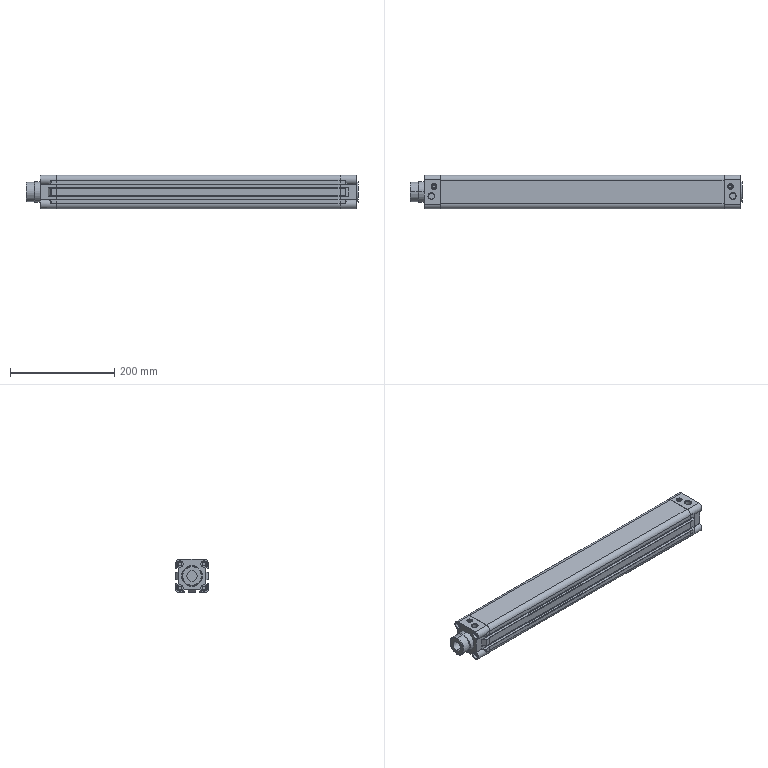Part | NX | features BREP 1 | 1 solid | 398 faces | box 636.5 x 64 x 64 mm | volume 1205229 mm3 | cylinder 190 | plane 176 | cone 30 | torus 2 | commonest cylinder face diameters 1 x102 6.647 x16 12.4 x16 17.5 x10 19 x10 20.2 x6